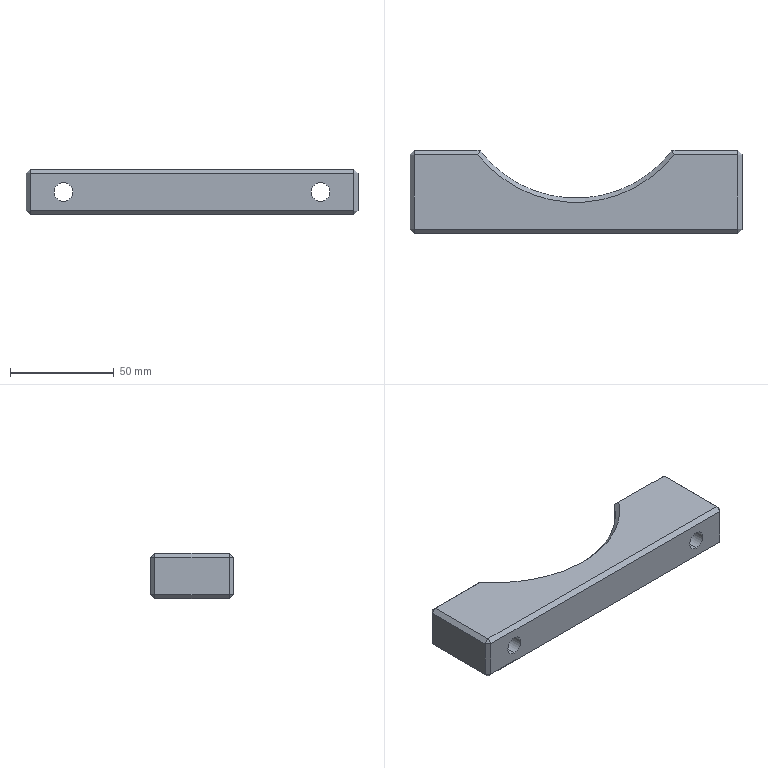Part | STEP file | Screw lock-middle support | 1 solid | 42 faces | box 160 x 40 x 22 mm | volume 96700 mm3 | plane 31 | cylinder 9 | cone 2 | commonest cylinder face diameters 9 x4 15 x4 116 x1